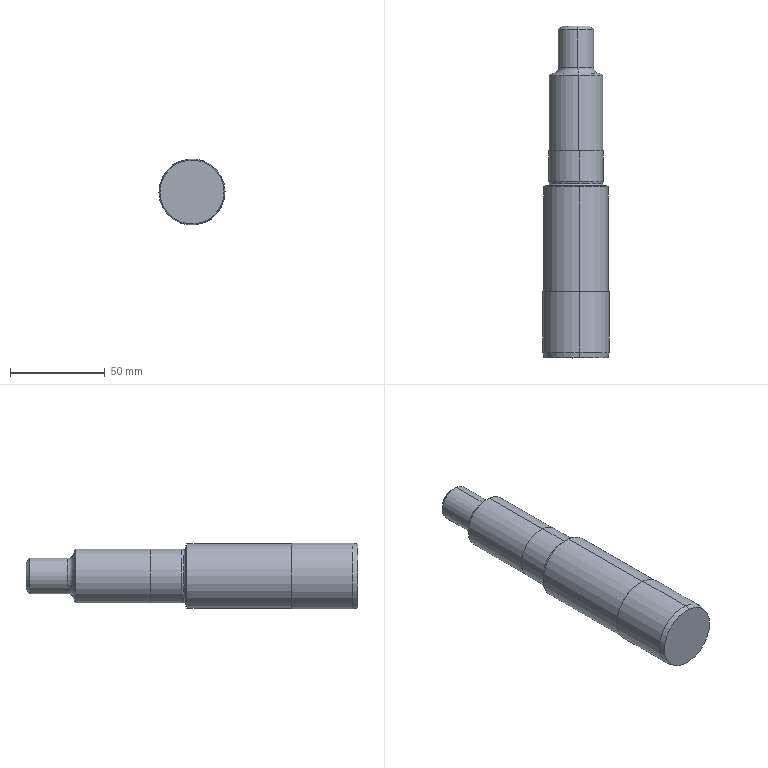Part | NX | features BREP 1 | 1 solid | 29 faces | box 34.96 x 175.503 x 34.96 mm | volume 129895 mm3 | cone 12 | cylinder 10 | plane 5 | torus 2 | commonest cylinder face diameters 18.77 x2 28.4 x2 28.619 x2 34.29 x2 34.96 x2
STEP:
#1=CARTESIAN_POINT('',(68.908,260.023,-25.976));
#2=VERTEX_POINT('',#1);
#3=CARTESIAN_POINT('',(66.192,260.023,-50.224));
#4=VERTEX_POINT('',#3);
#5=CARTESIAN_POINT('',(67.55,260.023,-38.1));
#6=DIRECTION('',(0.,1.,0.));
#7=DIRECTION('',(-0.1113,0.,-0.9938));
#8=AXIS2_PLACEMENT_3D('',#5,#6,#7);
#9=CIRCLE('',#8,12.2);
#10=EDGE_CURVE('',#2,#4,#9,.T.);
#11=ORIENTED_EDGE('',*,*,#10,.T.);
#12=CARTESIAN_POINT('',(66.505,263.017,-47.427));
#13=VERTEX_POINT('',#12);
#14=CARTESIAN_POINT('',(66.171,263.017,-50.408));
#15=DIRECTION('',(-0.9938,0.,0.1113));
#16=DIRECTION('',(0.1113,0.,0.9938));
#17=AXIS2_PLACEMENT_3D('',#14,#15,#16);
#18=CIRCLE('',#17,3.);
#19=EDGE_CURVE('',#4,#13,#18,.T.);
#20=ORIENTED_EDGE('',*,*,#19,.T.);
#21=CARTESIAN_POINT('',(68.595,263.017,-28.773));
#22=VERTEX_POINT('',#21);
#23=CARTESIAN_POINT('',(67.55,263.017,-38.1));
#24=DIRECTION('',(0.,1.,0.));
#25=DIRECTION('',(0.1113,0.,0.9938));
#26=AXIS2_PLACEMENT_3D('',#23,#24,#25);
#27=CIRCLE('',#26,9.385);
#28=EDGE_CURVE('',#22,#13,#27,.T.);
#29=ORIENTED_EDGE('',*,*,#28,.F.);
#30=CARTESIAN_POINT('',(68.929,263.017,-25.792));
#31=DIRECTION('',(0.9938,0.,-0.1113));
#32=DIRECTION('',(-0.1113,0.,-0.9938));
#33=AXIS2_PLACEMENT_3D('',#30,#31,#32);
#34=CIRCLE('',#33,3.);
#35=EDGE_CURVE('',#2,#22,#34,.T.);
#36=ORIENTED_EDGE('',*,*,#35,.F.);
#37=EDGE_LOOP('',(#11,#20,#29,#36));
#38=FACE_BOUND('',#37,.T.);
#39=CARTESIAN_POINT('',(67.55,263.017,-38.1));
#40=DIRECTION('',(0.,-1.,0.));
#41=DIRECTION('',(-0.1113,0.,-0.9938));
#42=AXIS2_PLACEMENT_3D('',#39,#40,#41);
#43=TOROIDAL_SURFACE('',#42,12.385,3.);
#44=ADVANCED_FACE('',(#38),#43,.F.);
#45=CARTESIAN_POINT('',(67.55,260.023,-38.1));
#46=DIRECTION('',(0.,1.,0.));
#47=DIRECTION('',(-0.1113,0.,-0.9938));
#48=AXIS2_PLACEMENT_3D('',#45,#46,#47);
#49=CIRCLE('',#48,12.2);
#50=EDGE_CURVE('',#4,#2,#49,.T.);
#51=ORIENTED_EDGE('',*,*,#50,.F.);
#52=CARTESIAN_POINT('',(65.969,258.868,-52.212));
#53=VERTEX_POINT('',#52);
#54=CARTESIAN_POINT('',(66.192,260.023,-50.224));
#55=DIRECTION('',(-0.0964,-0.5,-0.8606));
#56=VECTOR('',#55,1000.);
#57=LINE('',#54,#56);
#58=EDGE_CURVE('',#4,#53,#57,.T.);
#59=ORIENTED_EDGE('',*,*,#58,.T.);
#60=CARTESIAN_POINT('',(69.131,258.868,-23.988));
#61=VERTEX_POINT('',#60);
#62=CARTESIAN_POINT('',(67.55,258.868,-38.1));
#63=DIRECTION('',(0.,-1.,0.));
#64=DIRECTION('',(-0.1113,0.,-0.9938));
#65=AXIS2_PLACEMENT_3D('',#62,#63,#64);
#66=CIRCLE('',#65,14.2);
#67=EDGE_CURVE('',#61,#53,#66,.T.);
#68=ORIENTED_EDGE('',*,*,#67,.F.);
#69=CARTESIAN_POINT('',(68.908,260.023,-25.976));
#70=DIRECTION('',(0.0964,-0.5,0.8606));
#71=VECTOR('',#70,1000.);
#72=LINE('',#69,#71);
#73=EDGE_CURVE('',#2,#61,#72,.T.);
#74=ORIENTED_EDGE('',*,*,#73,.F.);
#75=EDGE_LOOP('',(#51,#59,#68,#74));
#76=FACE_BOUND('',#75,.T.);
#77=CARTESIAN_POINT('',(67.55,260.023,-38.1));
#78=DIRECTION('',(0.,-1.,0.));
#79=DIRECTION('',(-0.1113,0.,-0.9938));
#80=AXIS2_PLACEMENT_3D('',#77,#78,#79);
#81=CONICAL_SURFACE('',#80,12.2,1.047);
#82=ADVANCED_FACE('',(#76),#81,.T.);
#83=CARTESIAN_POINT('',(65.753,200.52,-54.145));
#84=VERTEX_POINT('',#83);
#85=CARTESIAN_POINT('',(69.347,200.52,-22.055));
#86=VERTEX_POINT('',#85);
#87=CARTESIAN_POINT('',(67.55,200.52,-38.1));
#88=DIRECTION('',(0.,1.,0.));
#89=DIRECTION('',(-0.1113,0.,-0.9938));
#90=AXIS2_PLACEMENT_3D('',#87,#88,#89);
#91=CIRCLE('',#90,16.145);
#92=EDGE_CURVE('',#84,#86,#91,.T.);
#93=ORIENTED_EDGE('',*,*,#92,.F.);
#94=CARTESIAN_POINT('',(65.642,199.943,-55.138));
#95=VERTEX_POINT('',#94);
#96=CARTESIAN_POINT('',(65.753,200.52,-54.145));
#97=DIRECTION('',(-0.0964,-0.5,-0.8606));
#98=VECTOR('',#97,1000.);
#99=LINE('',#96,#98);
#100=EDGE_CURVE('',#84,#95,#99,.T.);
#101=ORIENTED_EDGE('',*,*,#100,.T.);
#102=CARTESIAN_POINT('',(69.458,199.943,-21.062));
#103=VERTEX_POINT('',#102);
#104=CARTESIAN_POINT('',(67.55,199.943,-38.1));
#105=DIRECTION('',(0.,-1.,0.));
#106=DIRECTION('',(-0.1113,0.,-0.9938));
#107=AXIS2_PLACEMENT_3D('',#104,#105,#106);
#108=CIRCLE('',#107,17.145);
#109=EDGE_CURVE('',#103,#95,#108,.T.);
#110=ORIENTED_EDGE('',*,*,#109,.F.);
#111=CARTESIAN_POINT('',(69.347,200.52,-22.055));
#112=DIRECTION('',(0.0964,-0.5,0.8606));
#113=VECTOR('',#112,1000.);
#114=LINE('',#111,#113);
#115=EDGE_CURVE('',#86,#103,#114,.T.);
#116=ORIENTED_EDGE('',*,*,#115,.F.);
#117=EDGE_LOOP('',(#93,#101,#110,#116));
#118=FACE_BOUND('',#117,.T.);
#119=CARTESIAN_POINT('',(67.55,200.52,-38.1));
#120=DIRECTION('',(0.,-1.,0.));
#121=DIRECTION('',(-0.1113,0.,-0.9938));
#122=AXIS2_PLACEMENT_3D('',#119,#120,#121);
#123=CONICAL_SURFACE('',#122,16.145,1.047);
#124=ADVANCED_FACE('',(#118),#123,.T.);
#125=CARTESIAN_POINT('',(66.728,285.023,-45.439));
#126=VERTEX_POINT('',#125);
#127=CARTESIAN_POINT('',(68.372,285.023,-30.761));
#128=VERTEX_POINT('',#127);
#129=CARTESIAN_POINT('',(67.55,285.023,-38.1));
#130=DIRECTION('',(0.,1.,0.));
#131=DIRECTION('',(-0.1113,0.,-0.9938));
#132=AXIS2_PLACEMENT_3D('',#129,#130,#131);
#133=CIRCLE('',#132,7.385);
#134=EDGE_CURVE('',#126,#128,#133,.T.);
#135=ORIENTED_EDGE('',*,*,#134,.F.);
#136=CARTESIAN_POINT('',(66.505,283.023,-47.427));
#137=VERTEX_POINT('',#136);
#138=CARTESIAN_POINT('',(66.728,285.023,-45.439));
#139=DIRECTION('',(-0.07871,-0.7071,-0.7027));
#140=VECTOR('',#139,1000.);
#141=LINE('',#138,#140);
#142=EDGE_CURVE('',#126,#137,#141,.T.);
#143=ORIENTED_EDGE('',*,*,#142,.T.);
#144=CARTESIAN_POINT('',(68.595,283.023,-28.773));
#145=VERTEX_POINT('',#144);
#146=CARTESIAN_POINT('',(67.55,283.023,-38.1));
#147=DIRECTION('',(0.,-1.,0.));
#148=DIRECTION('',(-0.1113,0.,-0.9938));
#149=AXIS2_PLACEMENT_3D('',#146,#147,#148);
#150=CIRCLE('',#149,9.385);
#151=EDGE_CURVE('',#145,#137,#150,.T.);
#152=ORIENTED_EDGE('',*,*,#151,.F.);
#153=CARTESIAN_POINT('',(68.372,285.023,-30.761));
#154=DIRECTION('',(0.07871,-0.7071,0.7027));
#155=VECTOR('',#154,1000.);
#156=LINE('',#153,#155);
#157=EDGE_CURVE('',#128,#145,#156,.T.);
#158=ORIENTED_EDGE('',*,*,#157,.F.);
#159=EDGE_LOOP('',(#135,#143,#152,#158));
#160=FACE_BOUND('',#159,.T.);
#161=CARTESIAN_POINT('',(67.55,285.023,-38.1));
#162=DIRECTION('',(0.,-1.,0.));
#163=DIRECTION('',(-0.1113,0.,-0.9938));
#164=AXIS2_PLACEMENT_3D('',#161,#162,#163);
#165=CONICAL_SURFACE('',#164,7.385,0.7854);
#166=ADVANCED_FACE('',(#160),#165,.T.);
#167=ORIENTED_EDGE('',*,*,#151,.T.);
#168=CARTESIAN_POINT('',(66.505,285.023,-47.427));
#169=DIRECTION('',(0.,-1.,0.));
#170=VECTOR('',#169,1000.);
#171=LINE('',#168,#170);
#172=EDGE_CURVE('',#137,#13,#171,.T.);
#173=ORIENTED_EDGE('',*,*,#172,.T.);
#174=CARTESIAN_POINT('',(67.55,263.017,-38.1));
#175=DIRECTION('',(0.,1.,0.));
#176=DIRECTION('',(0.1113,0.,0.9938));
#177=AXIS2_PLACEMENT_3D('',#174,#175,#176);
#178=CIRCLE('',#177,9.385);
#179=EDGE_CURVE('',#13,#22,#178,.T.);
#180=ORIENTED_EDGE('',*,*,#179,.T.);
#181=CARTESIAN_POINT('',(68.595,285.023,-28.773));
#182=DIRECTION('',(0.,-1.,0.));
#183=VECTOR('',#182,1000.);
#184=LINE('',#181,#183);
#185=EDGE_CURVE('',#145,#22,#184,.T.);
#186=ORIENTED_EDGE('',*,*,#185,.F.);
#187=EDGE_LOOP('',(#167,#173,#180,#186));
#188=FACE_BOUND('',#187,.T.);
#189=CARTESIAN_POINT('',(67.55,285.023,-38.1));
#190=DIRECTION('',(0.,-1.,0.));
#191=DIRECTION('',(-0.1113,0.,-0.9938));
#192=AXIS2_PLACEMENT_3D('',#189,#190,#191);
#193=CYLINDRICAL_SURFACE('',#192,9.385);
#194=ADVANCED_FACE('',(#188),#193,.T.);
#195=ORIENTED_EDGE('',*,*,#67,.T.);
#196=CARTESIAN_POINT('',(65.969,219.023,-52.212));
#197=VERTEX_POINT('',#196);
#198=CARTESIAN_POINT('',(65.969,260.023,-52.212));
#199=DIRECTION('',(0.,-1.,0.));
#200=VECTOR('',#199,1000.);
#201=LINE('',#198,#200);
#202=EDGE_CURVE('',#53,#197,#201,.T.);
#203=ORIENTED_EDGE('',*,*,#202,.T.);
#204=CARTESIAN_POINT('',(69.131,219.023,-23.988));
#205=VERTEX_POINT('',#204);
#206=CARTESIAN_POINT('',(67.55,219.023,-38.1));
#207=DIRECTION('',(0.,1.,0.));
#208=DIRECTION('',(-0.1113,0.,-0.9938));
#209=AXIS2_PLACEMENT_3D('',#206,#207,#208);
#210=CIRCLE('',#209,14.2);
#211=EDGE_CURVE('',#197,#205,#210,.T.);
#212=ORIENTED_EDGE('',*,*,#211,.T.);
#213=CARTESIAN_POINT('',(69.131,260.023,-23.988));
#214=DIRECTION('',(0.,-1.,0.));
#215=VECTOR('',#214,1000.);
#216=LINE('',#213,#215);
#217=EDGE_CURVE('',#61,#205,#216,.T.);
#218=ORIENTED_EDGE('',*,*,#217,.F.);
#219=EDGE_LOOP('',(#195,#203,#212,#218));
#220=FACE_BOUND('',#219,.T.);
#221=CARTESIAN_POINT('',(67.55,260.023,-38.1));
#222=DIRECTION('',(0.,-1.,0.));
#223=DIRECTION('',(-0.1113,0.,-0.9938));
#224=AXIS2_PLACEMENT_3D('',#221,#222,#223);
#225=CYLINDRICAL_SURFACE('',#224,14.2);
#226=ADVANCED_FACE('',(#220),#225,.T.);
#227=CARTESIAN_POINT('',(65.957,219.023,-52.321));
#228=VERTEX_POINT('',#227);
#229=CARTESIAN_POINT('',(69.143,219.023,-23.879));
#230=VERTEX_POINT('',#229);
#231=CARTESIAN_POINT('',(67.55,219.023,-38.1));
#232=DIRECTION('',(0.,1.,0.));
#233=DIRECTION('',(-0.1113,0.,-0.9938));
#234=AXIS2_PLACEMENT_3D('',#231,#232,#233);
#235=CIRCLE('',#234,14.31);
#236=EDGE_CURVE('',#228,#230,#235,.T.);
#237=ORIENTED_EDGE('',*,*,#236,.F.);
#238=CARTESIAN_POINT('',(65.957,202.723,-52.321));
#239=VERTEX_POINT('',#238);
#240=CARTESIAN_POINT('',(65.957,219.023,-52.321));
#241=DIRECTION('',(0.,-1.,0.));
#242=VECTOR('',#241,1000.);
#243=LINE('',#240,#242);
#244=EDGE_CURVE('',#228,#239,#243,.T.);
#245=ORIENTED_EDGE('',*,*,#244,.T.);
#246=CARTESIAN_POINT('',(69.143,202.723,-23.879));
#247=VERTEX_POINT('',#246);
#248=CARTESIAN_POINT('',(67.55,202.723,-38.1));
#249=DIRECTION('',(0.,1.,0.));
#250=DIRECTION('',(-0.1113,0.,-0.9938));
#251=AXIS2_PLACEMENT_3D('',#248,#249,#250);
#252=CIRCLE('',#251,14.31);
#253=EDGE_CURVE('',#239,#247,#252,.T.);
#254=ORIENTED_EDGE('',*,*,#253,.T.);
#255=CARTESIAN_POINT('',(69.143,219.023,-23.879));
#256=DIRECTION('',(0.,-1.,0.));
#257=VECTOR('',#256,1000.);
#258=LINE('',#255,#257);
#259=EDGE_CURVE('',#230,#247,#258,.T.);
#260=ORIENTED_EDGE('',*,*,#259,.F.);
#261=EDGE_LOOP('',(#237,#245,#254,#260));
#262=FACE_BOUND('',#261,.T.);
#263=CARTESIAN_POINT('',(67.55,219.023,-38.1));
#264=DIRECTION('',(0.,-1.,0.));
#265=DIRECTION('',(-0.1113,0.,-0.9938));
#266=AXIS2_PLACEMENT_3D('',#263,#264,#265);
#267=CYLINDRICAL_SURFACE('',#266,14.31);
#268=ADVANCED_FACE('',(#262),#267,.T.);
#269=CARTESIAN_POINT('',(65.993,201.53,-52.003));
#270=VERTEX_POINT('',#269);
#271=CARTESIAN_POINT('',(69.107,201.53,-24.197));
#272=VERTEX_POINT('',#271);
#273=CARTESIAN_POINT('',(67.55,201.53,-38.1));
#274=DIRECTION('',(0.,1.,0.));
#275=DIRECTION('',(-0.1113,0.,-0.9938));
#276=AXIS2_PLACEMENT_3D('',#273,#274,#275);
#277=CIRCLE('',#276,13.99);
#278=EDGE_CURVE('',#270,#272,#277,.T.);
#279=ORIENTED_EDGE('',*,*,#278,.T.);
#280=CARTESIAN_POINT('',(69.107,201.53,-24.197));
#281=DIRECTION('',(0.02881,0.9659,0.2572));
#282=VECTOR('',#281,1000.);
#283=LINE('',#280,#282);
#284=EDGE_CURVE('',#247,#272,#283,.F.);
#285=ORIENTED_EDGE('',*,*,#284,.F.);
#286=ORIENTED_EDGE('',*,*,#253,.F.);
#287=CARTESIAN_POINT('',(65.993,201.53,-52.003));
#288=DIRECTION('',(-0.02881,0.9659,-0.2572));
#289=VECTOR('',#288,1000.);
#290=LINE('',#287,#289);
#291=EDGE_CURVE('',#239,#270,#290,.F.);
#292=ORIENTED_EDGE('',*,*,#291,.T.);
#293=EDGE_LOOP('',(#279,#285,#286,#292));
#294=FACE_BOUND('',#293,.T.);
#295=CARTESIAN_POINT('',(67.55,201.53,-38.1));
#296=DIRECTION('',(0.,1.,0.));
#297=DIRECTION('',(0.1113,0.,0.9938));
#298=AXIS2_PLACEMENT_3D('',#295,#296,#297);
#299=CONICAL_SURFACE('',#298,13.99,0.2618);
#300=ADVANCED_FACE('',(#294),#299,.T.);
#301=CARTESIAN_POINT('',(67.55,201.53,-38.1));
#302=DIRECTION('',(0.,1.,0.));
#303=DIRECTION('',(-0.1113,0.,-0.9938));
#304=AXIS2_PLACEMENT_3D('',#301,#302,#303);
#305=CIRCLE('',#304,13.99);
#306=EDGE_CURVE('',#272,#270,#305,.T.);
#307=ORIENTED_EDGE('',*,*,#306,.F.);
#308=CARTESIAN_POINT('',(69.22,200.52,-23.193));
#309=VERTEX_POINT('',#308);
#310=CARTESIAN_POINT('',(69.22,200.52,-23.193));
#311=DIRECTION('',(0.07871,-0.7071,0.7027));
#312=VECTOR('',#311,1000.);
#313=LINE('',#310,#312);
#314=EDGE_CURVE('',#309,#272,#313,.F.);
#315=ORIENTED_EDGE('',*,*,#314,.F.);
#316=CARTESIAN_POINT('',(65.88,200.52,-53.007));
#317=VERTEX_POINT('',#316);
#318=CARTESIAN_POINT('',(67.55,200.52,-38.1));
#319=DIRECTION('',(0.,1.,0.));
#320=DIRECTION('',(-0.1113,0.,-0.9938));
#321=AXIS2_PLACEMENT_3D('',#318,#319,#320);
#322=CIRCLE('',#321,15.);
#323=EDGE_CURVE('',#309,#317,#322,.T.);
#324=ORIENTED_EDGE('',*,*,#323,.T.);
#325=CARTESIAN_POINT('',(65.88,200.52,-53.007));
#326=DIRECTION('',(-0.07871,-0.7071,-0.7027));
#327=VECTOR('',#326,1000.);
#328=LINE('',#325,#327);
#329=EDGE_CURVE('',#317,#270,#328,.F.);
#330=ORIENTED_EDGE('',*,*,#329,.T.);
#331=EDGE_LOOP('',(#307,#315,#324,#330));
#332=FACE_BOUND('',#331,.T.);
#333=CARTESIAN_POINT('',(67.55,200.52,-38.1));
#334=DIRECTION('',(0.,-1.,0.));
#335=DIRECTION('',(0.1113,0.,0.9938));
#336=AXIS2_PLACEMENT_3D('',#333,#334,#335);
#337=CONICAL_SURFACE('',#336,15.,0.7854);
#338=ADVANCED_FACE('',(#332),#337,.T.);
#339=ORIENTED_EDGE('',*,*,#109,.T.);
#340=CARTESIAN_POINT('',(65.642,144.52,-55.138));
#341=VERTEX_POINT('',#340);
#342=CARTESIAN_POINT('',(65.642,200.52,-55.138));
#343=DIRECTION('',(0.,-1.,0.));
#344=VECTOR('',#343,1000.);
#345=LINE('',#342,#344);
#346=EDGE_CURVE('',#95,#341,#345,.T.);
#347=ORIENTED_EDGE('',*,*,#346,.T.);
#348=CARTESIAN_POINT('',(69.458,144.52,-21.062));
#349=VERTEX_POINT('',#348);
#350=CARTESIAN_POINT('',(67.55,144.52,-38.1));
#351=DIRECTION('',(0.,1.,0.));
#352=DIRECTION('',(-0.1113,0.,-0.9938));
#353=AXIS2_PLACEMENT_3D('',#350,#351,#352);
#354=CIRCLE('',#353,17.145);
#355=EDGE_CURVE('',#341,#349,#354,.T.);
#356=ORIENTED_EDGE('',*,*,#355,.T.);
#357=CARTESIAN_POINT('',(69.458,200.52,-21.062));
#358=DIRECTION('',(0.,-1.,0.));
#359=VECTOR('',#358,1000.);
#360=LINE('',#357,#359);
#361=EDGE_CURVE('',#103,#349,#360,.T.);
#362=ORIENTED_EDGE('',*,*,#361,.F.);
#363=EDGE_LOOP('',(#339,#347,#356,#362));
#364=FACE_BOUND('',#363,.T.);
#365=CARTESIAN_POINT('',(67.55,200.52,-38.1));
#366=DIRECTION('',(0.,-1.,0.));
#367=DIRECTION('',(-0.1113,0.,-0.9938));
#368=AXIS2_PLACEMENT_3D('',#365,#366,#367);
#369=CYLINDRICAL_SURFACE('',#368,17.145);
#370=ADVANCED_FACE('',(#364),#369,.T.);
#371=CARTESIAN_POINT('',(65.604,144.52,-55.471));
#372=VERTEX_POINT('',#371);
#373=CARTESIAN_POINT('',(69.496,144.52,-20.729));
#374=VERTEX_POINT('',#373);
#375=CARTESIAN_POINT('',(67.55,144.52,-38.1));
#376=DIRECTION('',(0.,1.,0.));
#377=DIRECTION('',(-0.1113,0.,-0.9938));
#378=AXIS2_PLACEMENT_3D('',#375,#376,#377);
#379=CIRCLE('',#378,17.48);
#380=EDGE_CURVE('',#372,#374,#379,.T.);
#381=ORIENTED_EDGE('',*,*,#380,.F.);
#382=CARTESIAN_POINT('',(65.604,112.62,-55.471));
#383=VERTEX_POINT('',#382);
#384=CARTESIAN_POINT('',(65.604,144.52,-55.471));
#385=DIRECTION('',(0.,-1.,0.));
#386=VECTOR('',#385,1000.);
#387=LINE('',#384,#386);
#388=EDGE_CURVE('',#372,#383,#387,.T.);
#389=ORIENTED_EDGE('',*,*,#388,.T.);
#390=CARTESIAN_POINT('',(69.496,112.62,-20.729));
#391=VERTEX_POINT('',#390);
#392=CARTESIAN_POINT('',(67.55,112.62,-38.1));
#393=DIRECTION('',(0.,1.,0.));
#394=DIRECTION('',(-0.1113,0.,-0.9938));
#395=AXIS2_PLACEMENT_3D('',#392,#393,#394);
#396=CIRCLE('',#395,17.48);
#397=EDGE_CURVE('',#383,#391,#396,.T.);
#398=ORIENTED_EDGE('',*,*,#397,.T.);
#399=CARTESIAN_POINT('',(69.496,144.52,-20.729));
#400=DIRECTION('',(0.,-1.,0.));
#401=VECTOR('',#400,1000.);
#402=LINE('',#399,#401);
#403=EDGE_CURVE('',#374,#391,#402,.T.);
#404=ORIENTED_EDGE('',*,*,#403,.F.);
#405=EDGE_LOOP('',(#381,#389,#398,#404));
#406=FACE_BOUND('',#405,.T.);
#407=CARTESIAN_POINT('',(67.55,144.52,-38.1));
#408=DIRECTION('',(0.,-1.,0.));
#409=DIRECTION('',(-0.1113,0.,-0.9938));
#410=AXIS2_PLACEMENT_3D('',#407,#408,#409);
#411=CYLINDRICAL_SURFACE('',#410,17.48);
#412=ADVANCED_FACE('',(#406),#411,.T.);
#413=CARTESIAN_POINT('',(69.435,109.52,-21.272));
#414=VERTEX_POINT('',#413);
#415=CARTESIAN_POINT('',(65.665,109.52,-54.928));
#416=VERTEX_POINT('',#415);
#417=CARTESIAN_POINT('',(67.55,109.52,-38.1));
#418=DIRECTION('',(0.,-1.,0.));
#419=DIRECTION('',(-1.,0.,0.));
#420=AXIS2_PLACEMENT_3D('',#417,#418,#419);
#421=CIRCLE('',#420,16.933);
#422=EDGE_CURVE('',#414,#416,#421,.T.);
#423=ORIENTED_EDGE('',*,*,#422,.F.);
#424=CARTESIAN_POINT('',(69.496,112.62,-20.729));
#425=DIRECTION('',(0.01933,0.9848,0.1726));
#426=VECTOR('',#425,1000.);
#427=LINE('',#424,#426);
#428=EDGE_CURVE('',#391,#414,#427,.F.);
#429=ORIENTED_EDGE('',*,*,#428,.F.);
#430=ORIENTED_EDGE('',*,*,#397,.F.);
#431=CARTESIAN_POINT('',(65.604,112.62,-55.471));
#432=DIRECTION('',(-0.01933,0.9848,-0.1726));
#433=VECTOR('',#432,1000.);
#434=LINE('',#431,#433);
#435=EDGE_CURVE('',#383,#416,#434,.F.);
#436=ORIENTED_EDGE('',*,*,#435,.T.);
#437=EDGE_LOOP('',(#423,#429,#430,#436));
#438=FACE_BOUND('',#437,.T.);
#439=CARTESIAN_POINT('',(67.55,112.62,-38.1));
#440=DIRECTION('',(0.,1.,0.));
#441=DIRECTION('',(0.1113,0.,0.9938));
#442=AXIS2_PLACEMENT_3D('',#439,#440,#441);
#443=CONICAL_SURFACE('',#442,17.48,0.1745);
#444=ADVANCED_FACE('',(#438),#443,.T.);
#445=ORIENTED_EDGE('',*,*,#428,.T.);
#446=CARTESIAN_POINT('',(67.55,109.52,-38.1));
#447=DIRECTION('',(0.,-1.,0.));
#448=DIRECTION('',(-1.,0.,0.));
#449=AXIS2_PLACEMENT_3D('',#446,#447,#448);
#450=CIRCLE('',#449,16.933);
#451=EDGE_CURVE('',#416,#414,#450,.T.);
#452=ORIENTED_EDGE('',*,*,#451,.F.);
#453=ORIENTED_EDGE('',*,*,#435,.F.);
#454=CARTESIAN_POINT('',(67.55,112.62,-38.1));
#455=DIRECTION('',(0.,1.,0.));
#456=DIRECTION('',(-0.1113,0.,-0.9938));
#457=AXIS2_PLACEMENT_3D('',#454,#455,#456);
#458=CIRCLE('',#457,17.48);
#459=EDGE_CURVE('',#391,#383,#458,.T.);
#460=ORIENTED_EDGE('',*,*,#459,.F.);
#461=EDGE_LOOP('',(#445,#452,#453,#460));
#462=FACE_BOUND('',#461,.T.);
#463=CARTESIAN_POINT('',(67.55,112.62,-38.1));
#464=DIRECTION('',(0.,1.,0.));
#465=DIRECTION('',(0.1113,0.,0.9938));
#466=AXIS2_PLACEMENT_3D('',#463,#464,#465);
#467=CONICAL_SURFACE('',#466,17.48,0.1745);
#468=ADVANCED_FACE('',(#462),#467,.T.);
#469=ORIENTED_EDGE('',*,*,#388,.F.);
#470=CARTESIAN_POINT('',(67.55,144.52,-38.1));
#471=DIRECTION('',(0.,1.,0.));
#472=DIRECTION('',(-0.1113,0.,-0.9938));
#473=AXIS2_PLACEMENT_3D('',#470,#471,#472);
#474=CIRCLE('',#473,17.48);
#475=EDGE_CURVE('',#374,#372,#474,.T.);
#476=ORIENTED_EDGE('',*,*,#475,.F.);
#477=ORIENTED_EDGE('',*,*,#403,.T.);
#478=ORIENTED_EDGE('',*,*,#459,.T.);
#479=EDGE_LOOP('',(#469,#476,#477,#478));
#480=FACE_BOUND('',#479,.T.);
#481=CARTESIAN_POINT('',(67.55,144.52,-38.1));
#482=DIRECTION('',(0.,-1.,0.));
#483=DIRECTION('',(-0.1113,0.,-0.9938));
#484=AXIS2_PLACEMENT_3D('',#481,#482,#483);
#485=CYLINDRICAL_SURFACE('',#484,17.48);
#486=ADVANCED_FACE('',(#480),#485,.T.);
#487=CARTESIAN_POINT('',(67.55,144.52,-38.1));
#488=DIRECTION('',(0.,1.,0.));
#489=DIRECTION('',(-0.1113,0.,-0.9938));
#490=AXIS2_PLACEMENT_3D('',#487,#488,#489);
#491=CIRCLE('',#490,17.145);
#492=EDGE_CURVE('',#349,#341,#491,.T.);
#493=ORIENTED_EDGE('',*,*,#492,.F.);
#494=ORIENTED_EDGE('',*,*,#355,.F.);
#495=EDGE_LOOP('',(#493,#494));
#496=FACE_BOUND('',#495,.T.);
#497=ORIENTED_EDGE('',*,*,#475,.T.);
#498=ORIENTED_EDGE('',*,*,#380,.T.);
#499=EDGE_LOOP('',(#497,#498));
#500=FACE_BOUND('',#499,.T.);
#501=CARTESIAN_POINT('',(67.55,144.52,-38.1));
#502=DIRECTION('',(0.,1.,0.));
#503=DIRECTION('',(0.1113,0.,0.9938));
#504=AXIS2_PLACEMENT_3D('',#501,#502,#503);
#505=PLANE('',#504);
#506=ADVANCED_FACE('',(#496,#500),#505,.T.);
#507=ORIENTED_EDGE('',*,*,#346,.F.);
#508=CARTESIAN_POINT('',(67.55,199.943,-38.1));
#509=DIRECTION('',(0.,-1.,0.));
#510=DIRECTION('',(-0.1113,0.,-0.9938));
#511=AXIS2_PLACEMENT_3D('',#508,#509,#510);
#512=CIRCLE('',#511,17.145);
#513=EDGE_CURVE('',#95,#103,#512,.T.);
#514=ORIENTED_EDGE('',*,*,#513,.T.);
#515=ORIENTED_EDGE('',*,*,#361,.T.);
#516=ORIENTED_EDGE('',*,*,#492,.T.);
#517=EDGE_LOOP('',(#507,#514,#515,#516));
#518=FACE_BOUND('',#517,.T.);
#519=CARTESIAN_POINT('',(67.55,200.52,-38.1));
#520=DIRECTION('',(0.,-1.,0.));
#521=DIRECTION('',(-0.1113,0.,-0.9938));
#522=AXIS2_PLACEMENT_3D('',#519,#520,#521);
#523=CYLINDRICAL_SURFACE('',#522,17.145);
#524=ADVANCED_FACE('',(#518),#523,.T.);
#525=CARTESIAN_POINT('',(67.55,200.52,-38.1));
#526=DIRECTION('',(0.,1.,0.));
#527=DIRECTION('',(-0.1113,0.,-0.9938));
#528=AXIS2_PLACEMENT_3D('',#525,#526,#527);
#529=CIRCLE('',#528,16.145);
#530=EDGE_CURVE('',#86,#84,#529,.T.);
#531=ORIENTED_EDGE('',*,*,#530,.T.);
#532=ORIENTED_EDGE('',*,*,#92,.T.);
#533=EDGE_LOOP('',(#531,#532));
#534=FACE_BOUND('',#533,.T.);
#535=CARTESIAN_POINT('',(67.55,200.52,-38.1));
#536=DIRECTION('',(0.,1.,0.));
#537=DIRECTION('',(-0.1113,0.,-0.9938));
#538=AXIS2_PLACEMENT_3D('',#535,#536,#537);
#539=CIRCLE('',#538,15.);
#540=EDGE_CURVE('',#317,#309,#539,.T.);
#541=ORIENTED_EDGE('',*,*,#540,.F.);
#542=ORIENTED_EDGE('',*,*,#323,.F.);
#543=EDGE_LOOP('',(#541,#542));
#544=FACE_BOUND('',#543,.T.);
#545=CARTESIAN_POINT('',(67.55,200.52,-38.1));
#546=DIRECTION('',(0.,1.,0.));
#547=DIRECTION('',(0.1113,0.,0.9938));
#548=AXIS2_PLACEMENT_3D('',#545,#546,#547);
#549=PLANE('',#548);
#550=ADVANCED_FACE('',(#534,#544),#549,.T.);
#551=ORIENTED_EDGE('',*,*,#314,.T.);
#552=ORIENTED_EDGE('',*,*,#278,.F.);
#553=ORIENTED_EDGE('',*,*,#329,.F.);
#554=ORIENTED_EDGE('',*,*,#540,.T.);
#555=EDGE_LOOP('',(#551,#552,#553,#554));
#556=FACE_BOUND('',#555,.T.);
#557=CARTESIAN_POINT('',(67.55,200.52,-38.1));
#558=DIRECTION('',(0.,-1.,0.));
#559=DIRECTION('',(0.1113,0.,0.9938));
#560=AXIS2_PLACEMENT_3D('',#557,#558,#559);
#561=CONICAL_SURFACE('',#560,15.,0.7854);
#562=ADVANCED_FACE('',(#556),#561,.T.);
#563=ORIENTED_EDGE('',*,*,#284,.T.);
#564=ORIENTED_EDGE('',*,*,#306,.T.);
#565=ORIENTED_EDGE('',*,*,#291,.F.);
#566=CARTESIAN_POINT('',(67.55,202.723,-38.1));
#567=DIRECTION('',(0.,1.,0.));
#568=DIRECTION('',(-0.1113,0.,-0.9938));
#569=AXIS2_PLACEMENT_3D('',#566,#567,#568);
#570=CIRCLE('',#569,14.31);
#571=EDGE_CURVE('',#247,#239,#570,.T.);
#572=ORIENTED_EDGE('',*,*,#571,.F.);
#573=EDGE_LOOP('',(#563,#564,#565,#572));
#574=FACE_BOUND('',#573,.T.);
#575=CARTESIAN_POINT('',(67.55,201.53,-38.1));
#576=DIRECTION('',(0.,1.,0.));
#577=DIRECTION('',(0.1113,0.,0.9938));
#578=AXIS2_PLACEMENT_3D('',#575,#576,#577);
#579=CONICAL_SURFACE('',#578,13.99,0.2618);
#580=ADVANCED_FACE('',(#574),#579,.T.);
#581=ORIENTED_EDGE('',*,*,#244,.F.);
#582=CARTESIAN_POINT('',(67.55,219.023,-38.1));
#583=DIRECTION('',(0.,1.,0.));
#584=DIRECTION('',(-0.1113,0.,-0.9938));
#585=AXIS2_PLACEMENT_3D('',#582,#583,#584);
#586=CIRCLE('',#585,14.31);
#587=EDGE_CURVE('',#230,#228,#586,.T.);
#588=ORIENTED_EDGE('',*,*,#587,.F.);
#589=ORIENTED_EDGE('',*,*,#259,.T.);
#590=ORIENTED_EDGE('',*,*,#571,.T.);
#591=EDGE_LOOP('',(#581,#588,#589,#590));
#592=FACE_BOUND('',#591,.T.);
#593=CARTESIAN_POINT('',(67.55,219.023,-38.1));
#594=DIRECTION('',(0.,-1.,0.));
#595=DIRECTION('',(-0.1113,0.,-0.9938));
#596=AXIS2_PLACEMENT_3D('',#593,#594,#595);
#597=CYLINDRICAL_SURFACE('',#596,14.31);
#598=ADVANCED_FACE('',(#592),#597,.T.);
#599=CARTESIAN_POINT('',(67.55,219.023,-38.1));
#600=DIRECTION('',(0.,1.,0.));
#601=DIRECTION('',(-0.1113,0.,-0.9938));
#602=AXIS2_PLACEMENT_3D('',#599,#600,#601);
#603=CIRCLE('',#602,14.2);
#604=EDGE_CURVE('',#205,#197,#603,.T.);
#605=ORIENTED_EDGE('',*,*,#604,.F.);
#606=ORIENTED_EDGE('',*,*,#211,.F.);
#607=EDGE_LOOP('',(#605,#606));
#608=FACE_BOUND('',#607,.T.);
#609=ORIENTED_EDGE('',*,*,#587,.T.);
#610=ORIENTED_EDGE('',*,*,#236,.T.);
#611=EDGE_LOOP('',(#609,#610));
#612=FACE_BOUND('',#611,.T.);
#613=CARTESIAN_POINT('',(67.55,219.023,-38.1));
#614=DIRECTION('',(0.,1.,0.));
#615=DIRECTION('',(0.1113,0.,0.9938));
#616=AXIS2_PLACEMENT_3D('',#613,#614,#615);
#617=PLANE('',#616);
#618=ADVANCED_FACE('',(#608,#612),#617,.T.);
#619=ORIENTED_EDGE('',*,*,#202,.F.);
#620=CARTESIAN_POINT('',(67.55,258.868,-38.1));
#621=DIRECTION('',(0.,-1.,0.));
#622=DIRECTION('',(-0.1113,0.,-0.9938));
#623=AXIS2_PLACEMENT_3D('',#620,#621,#622);
#624=CIRCLE('',#623,14.2);
#625=EDGE_CURVE('',#53,#61,#624,.T.);
#626=ORIENTED_EDGE('',*,*,#625,.T.);
#627=ORIENTED_EDGE('',*,*,#217,.T.);
#628=ORIENTED_EDGE('',*,*,#604,.T.);
#629=EDGE_LOOP('',(#619,#626,#627,#628));
#630=FACE_BOUND('',#629,.T.);
#631=CARTESIAN_POINT('',(67.55,260.023,-38.1));
#632=DIRECTION('',(0.,-1.,0.));
#633=DIRECTION('',(-0.1113,0.,-0.9938));
#634=AXIS2_PLACEMENT_3D('',#631,#632,#633);
#635=CYLINDRICAL_SURFACE('',#634,14.2);
#636=ADVANCED_FACE('',(#630),#635,.T.);
#637=ORIENTED_EDGE('',*,*,#172,.F.);
#638=CARTESIAN_POINT('',(67.55,283.023,-38.1));
#639=DIRECTION('',(0.,-1.,0.));
#640=DIRECTION('',(-0.1113,0.,-0.9938));
#641=AXIS2_PLACEMENT_3D('',#638,#639,#640);
#642=CIRCLE('',#641,9.385);
#643=EDGE_CURVE('',#137,#145,#642,.T.);
#644=ORIENTED_EDGE('',*,*,#643,.T.);
#645=ORIENTED_EDGE('',*,*,#185,.T.);
#646=ORIENTED_EDGE('',*,*,#28,.T.);
#647=EDGE_LOOP('',(#637,#644,#645,#646));
#648=FACE_BOUND('',#647,.T.);
#649=CARTESIAN_POINT('',(67.55,285.023,-38.1));
#650=DIRECTION('',(0.,-1.,0.));
#651=DIRECTION('',(-0.1113,0.,-0.9938));
#652=AXIS2_PLACEMENT_3D('',#649,#650,#651);
#653=CYLINDRICAL_SURFACE('',#652,9.385);
#654=ADVANCED_FACE('',(#648),#653,.T.);
#655=CARTESIAN_POINT('',(67.55,285.023,-38.1));
#656=DIRECTION('',(0.,1.,0.));
#657=DIRECTION('',(-0.1113,0.,-0.9938));
#658=AXIS2_PLACEMENT_3D('',#655,#656,#657);
#659=CIRCLE('',#658,7.385);
#660=EDGE_CURVE('',#128,#126,#659,.T.);
#661=ORIENTED_EDGE('',*,*,#660,.T.);
#662=ORIENTED_EDGE('',*,*,#134,.T.);
#663=EDGE_LOOP('',(#661,#662));
#664=FACE_BOUND('',#663,.T.);
#665=CARTESIAN_POINT('',(67.55,285.023,-38.1));
#666=DIRECTION('',(0.,1.,0.));
#667=DIRECTION('',(0.1113,0.,0.9938));
#668=AXIS2_PLACEMENT_3D('',#665,#666,#667);
#669=PLANE('',#668);
#670=ADVANCED_FACE('',(#664),#669,.T.);
#671=ORIENTED_EDGE('',*,*,#142,.F.);
#672=ORIENTED_EDGE('',*,*,#660,.F.);
#673=ORIENTED_EDGE('',*,*,#157,.T.);
#674=ORIENTED_EDGE('',*,*,#643,.F.);
#675=EDGE_LOOP('',(#671,#672,#673,#674));
#676=FACE_BOUND('',#675,.T.);
#677=CARTESIAN_POINT('',(67.55,285.023,-38.1));
#678=DIRECTION('',(0.,-1.,0.));
#679=DIRECTION('',(-0.1113,0.,-0.9938));
#680=AXIS2_PLACEMENT_3D('',#677,#678,#679);
#681=CONICAL_SURFACE('',#680,7.385,0.7854);
#682=ADVANCED_FACE('',(#676),#681,.T.);
#683=ORIENTED_EDGE('',*,*,#100,.F.);
#684=ORIENTED_EDGE('',*,*,#530,.F.);
#685=ORIENTED_EDGE('',*,*,#115,.T.);
#686=ORIENTED_EDGE('',*,*,#513,.F.);
#687=EDGE_LOOP('',(#683,#684,#685,#686));
#688=FACE_BOUND('',#687,.T.);
#689=CARTESIAN_POINT('',(67.55,200.52,-38.1));
#690=DIRECTION('',(0.,-1.,0.));
#691=DIRECTION('',(-0.1113,0.,-0.9938));
#692=AXIS2_PLACEMENT_3D('',#689,#690,#691);
#693=CONICAL_SURFACE('',#692,16.145,1.047);
#694=ADVANCED_FACE('',(#688),#693,.T.);
#695=ORIENTED_EDGE('',*,*,#58,.F.);
#696=ORIENTED_EDGE('',*,*,#10,.F.);
#697=ORIENTED_EDGE('',*,*,#73,.T.);
#698=ORIENTED_EDGE('',*,*,#625,.F.);
#699=EDGE_LOOP('',(#695,#696,#697,#698));
#700=FACE_BOUND('',#699,.T.);
#701=CARTESIAN_POINT('',(67.55,260.023,-38.1));
#702=DIRECTION('',(0.,-1.,0.));
#703=DIRECTION('',(-0.1113,0.,-0.9938));
#704=AXIS2_PLACEMENT_3D('',#701,#702,#703);
#705=CONICAL_SURFACE('',#704,12.2,1.047);
#706=ADVANCED_FACE('',(#700),#705,.T.);
#707=ORIENTED_EDGE('',*,*,#19,.F.);
#708=ORIENTED_EDGE('',*,*,#50,.T.);
#709=ORIENTED_EDGE('',*,*,#35,.T.);
#710=ORIENTED_EDGE('',*,*,#179,.F.);
#711=EDGE_LOOP('',(#707,#708,#709,#710));
#712=FACE_BOUND('',#711,.T.);
#713=CARTESIAN_POINT('',(67.55,263.017,-38.1));
#714=DIRECTION('',(0.,-1.,0.));
#715=DIRECTION('',(-0.1113,0.,-0.9938));
#716=AXIS2_PLACEMENT_3D('',#713,#714,#715);
#717=TOROIDAL_SURFACE('',#716,12.385,3.);
#718=ADVANCED_FACE('',(#712),#717,.F.);
#719=ORIENTED_EDGE('',*,*,#451,.T.);
#720=ORIENTED_EDGE('',*,*,#422,.T.);
#721=EDGE_LOOP('',(#719,#720));
#722=FACE_BOUND('',#721,.T.);
#723=CARTESIAN_POINT('',(67.55,109.52,-38.1));
#724=DIRECTION('',(0.,1.,0.));
#725=DIRECTION('',(0.1113,0.,0.9938));
#726=AXIS2_PLACEMENT_3D('',#723,#724,#725);
#727=PLANE('',#726);
#728=ADVANCED_FACE('',(#722),#727,.F.);
#729=CLOSED_SHELL('',(#44,#82,#124,#166,#194,#226,#268,#300,#338,#370,#412,#444,#468,#486,#506,#524,#550,#562,#580,#598,#618,#636,#654,#670,#682,#694,#706,#718,#728));
#730=MANIFOLD_SOLID_BREP('',#729);
#731=(LENGTH_UNIT()NAMED_UNIT(*)SI_UNIT(.MILLI.,.METRE.));
#732=UNCERTAINTY_MEASURE_WITH_UNIT(LENGTH_MEASURE(0.00001),#731,'','');
#733=(NAMED_UNIT(*)PLANE_ANGLE_UNIT()SI_UNIT($,.RADIAN.));
#734=(NAMED_UNIT(*)SI_UNIT($,.STERADIAN.)SOLID_ANGLE_UNIT());
#735=(GEOMETRIC_REPRESENTATION_CONTEXT(3)GLOBAL_UNCERTAINTY_ASSIGNED_CONTEXT((#732))GLOBAL_UNIT_ASSIGNED_CONTEXT((#731,#733,#734))REPRESENTATION_CONTEXT('',''));
#736=ADVANCED_BREP_SHAPE_REPRESENTATION('',(#730),#735);